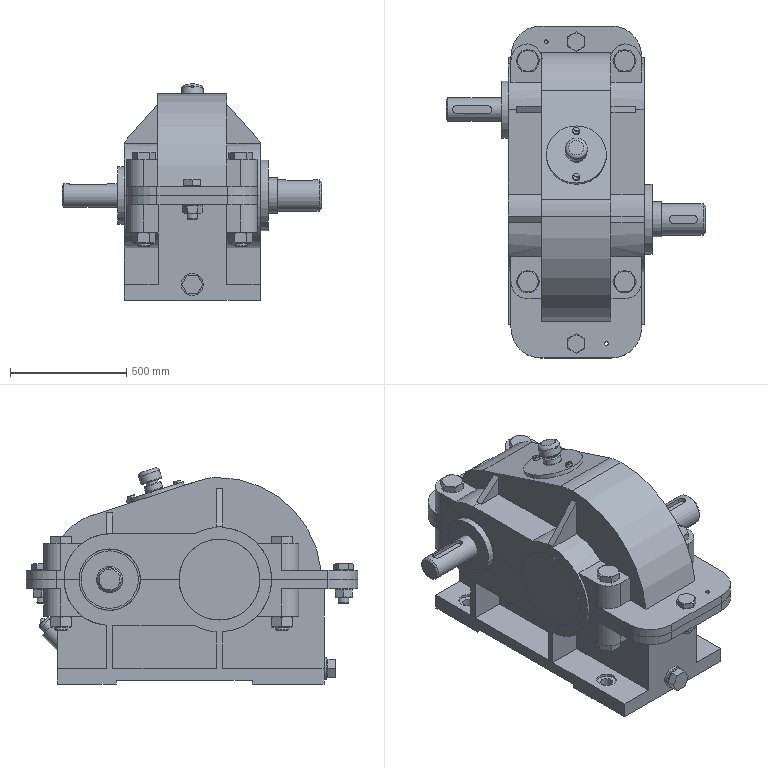Part | NX | features BREP 197, META 184, INSTANCE 70, Delete Body 36, LINKED_BODY 32, SKETCH 29, DATUM_CSYS 23, SCALE 22, CYLINDER 21, CHAMFER 16, BOSS 13, EXTRUDE 12, SIMPLE HOLE 10, UNITE 9, DATUM_PLANE 8, MOVE_FACE 8, SYMBOLIC_THREAD 8, SWP104 7, BLEND 5, REPLACE_FACE 5, SPLIT BODY 5, SUBTRACT 4, RECT_SLOT 3, 10.SLDPRT 2, 11.SLDPRT 2, 25.SLDPRT 2, 28.SLDPRT 2, 29.SLDPRT 2, 3.SLDPRT 2, 4.SLDPRT 2, 7.SLDPRT 2, CIRCULAR_ISET 2, EXTRACT_FACE 2, FSET 2, Resize Face 2, TRANSFORM_ISET 2, ABSOLUTE_DATUM_PLANE 1, Container 1, EXTRACT_BODY 1, Geometry Instance 1, Instance Feature 1, LINE 1, MIRROR 1, MIRROR_SET 1, Mirror Feature 1 | 39 solids | 2289 faces | volume 277364397 mm3 | spline 1120 | cylinder 446 | plane 417 | torus 147 | cone 98 | sphere 61 | commonest cylinder face diameters 765.703 x184 158.203 x40 264.375 x15 348.75 x14 84.375 x10 146.25 x10